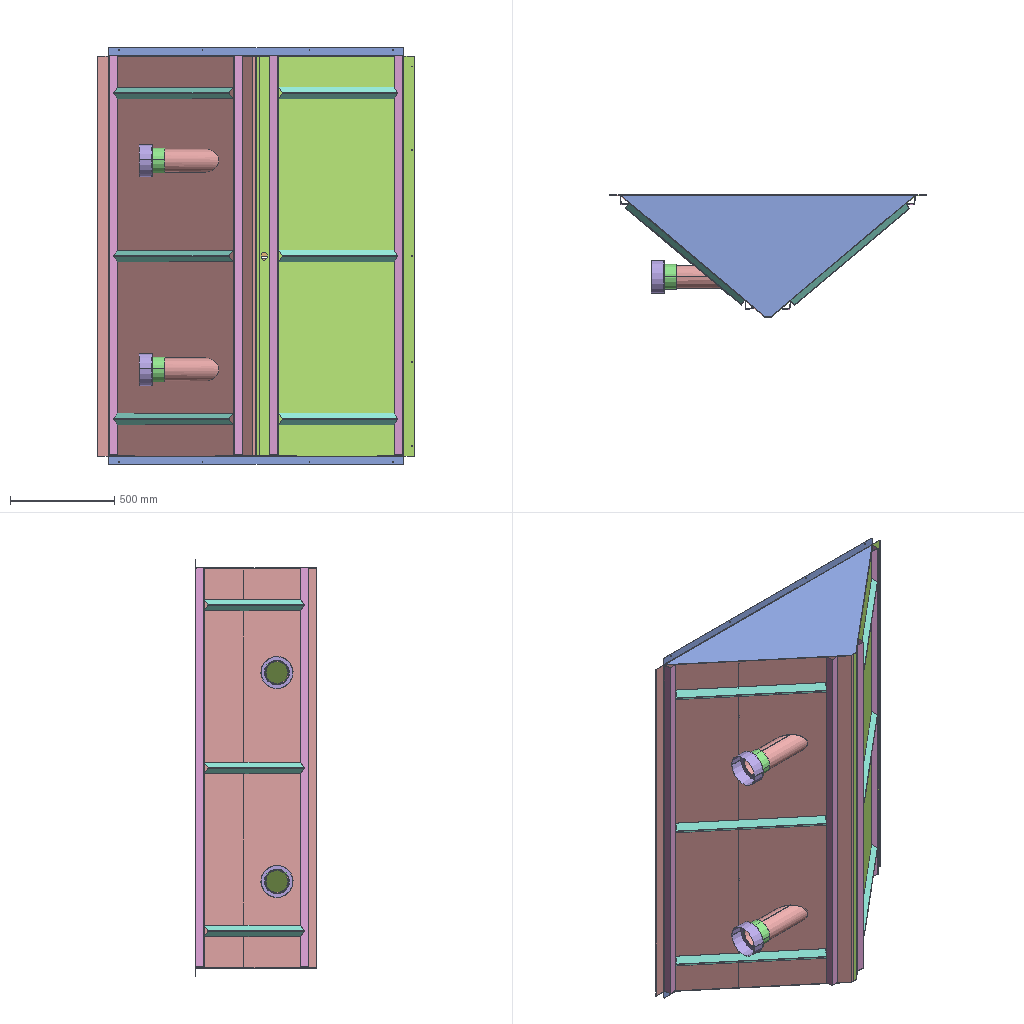Assembly | SolidWorks | 7 different items | 22 placed | box 1515 x 581 x 1994 mm
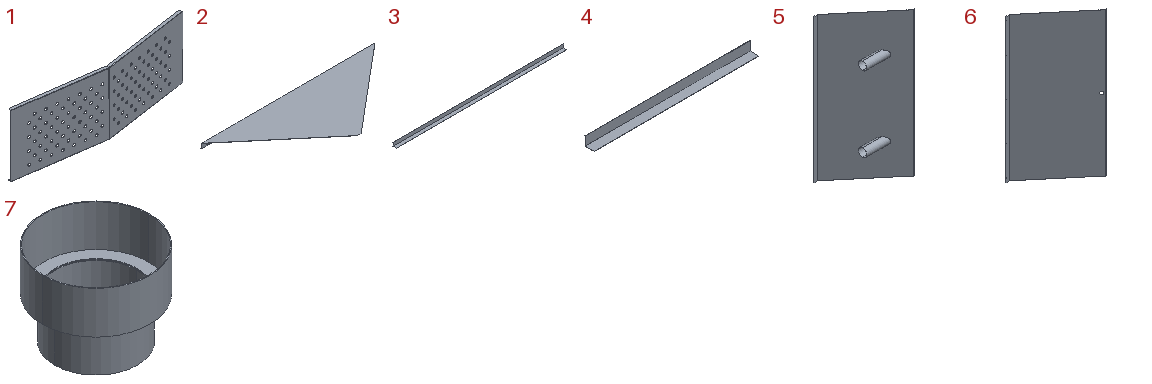Parts list (item | quantity | size | volume | features):
1 | x6 | 860.334 x 74.65 x 310 mm | 335938 mm3 | features LPattern 3, ICE 2, EdgeFlange 1, Fillet 1, FlatPattern 1, SMBaseFlange 1, SheetMetal 1
2 | x2 | 1412 x 580 x 40 mm | 567151 mm3 | features EdgeFlange 1, Fillet 1, FlatPattern 1, HoleWzd 1, SMBaseFlange 1, SheetMetal 1
3 | x4 | 1910 x 40 x 40 mm | 179921 mm3 | features EdgeFlange 1, FlatPattern 1, SMBaseFlange 1, SheetMetal 1
4 | x6 | 720 x 40 x 40 mm | 67824 mm3 | features EdgeFlange 1, FlatPattern 1, SMBaseFlange 1, SheetMetal 1
5 | x1 | 757 x 581.2 x 1915 mm | 2731991 mm3 | features ICE 2, FlatPattern 1, SMBaseFlange 1, SheetMetal 1
6 | x1 | 757 x 581.2 x 1915 mm | 2223001 mm3 | features FlatPattern 1, HoleWzd 1, ICE 1, SMBaseFlange 1, SheetMetal 1
7 | x2 | 155 x 155 x 121.2 mm | 70732 mm3 | features ICE 2, Extrusion 1
Mates (type | each side: item.copy, entity, surface, feature):
Coincident | 5.1 face plane Base-Flange1 | assembly face | 2 times
DistanceDim | 5.1 face plane Base-Flange1 | assembly face
Coincident | 5.1 face plane Base-Flange1 | 2.1 face plane Edge-Flange1
Coincident | 5.1 face plane Base-Flange1 | 2.2 face plane Base-Flange1
Coincident | 5.1 face plane Base-Flange1 | 6.1 face plane Base-Flange1 | 2 times
DistanceDim | 5.1 face plane Base-Flange1 | 6.1 face plane Base-Flange1
Width | 2.1 face plane Base-Flange1 | 2.1 face plane Base-Flange1 | 6.1 face plane Base-Flange1 | 5.1 face plane Base-Flange1
Coincident | 5.1 face plane Base-Flange1 | 2.1 face plane Base-Flange1
Coincident | 2.1 face plane Edge-Flange1 | 2.2 face plane Edge-Flange1 | 2 times
Coincident | 2.2 face plane Base-Flange1 | 3.1 face plane Base-Flange1
Coincident | 6.1 face plane Base-Flange1 | 3.1 edge | 2 times
Coincident | 5.1 face plane Base-Flange1 | 3.2 edge | 2 times
Coincident | 3.1 face plane Edge-Flange1 | 3.2 face plane Base-Flange1
Coincident | 6.1 face plane Base-Flange1 | 4.1 edge | 2 times
DistanceDim | 4.1 edge | 2.2 face plane Base-Flange1
Coincident | 5.1 face plane Base-Flange1 | 4.2 edge | 2 times
DistanceDim | 4.2 edge | 2.2 face plane Base-Flange1
Coincident | 2.1 face plane Base-Flange1 | 1.1 face plane Edge-Flange1
Width | 1.1 face plane Base-Flange1 | 1.1 face plane Base-Flange1 | 6.1 face plane Base-Flange1 | 5.1 face plane Base-Flange1
Coincident | 6.1 face plane Base-Flange1 | 1.1 edge
Concentric | 5.1 face cylinder Boss-Extrude1 | 7.1 face cylinder Boss-Extrude3
Coincident | 5.1 edge | 7.1 face plane Boss-Extrude2
Concentric | 5.1 face cylinder Boss-Extrude1 | 7.2 face cylinder Boss-Extrude3
Coincident | 7.1 face plane Boss-Extrude2 | 7.2 face plane Boss-Extrude2